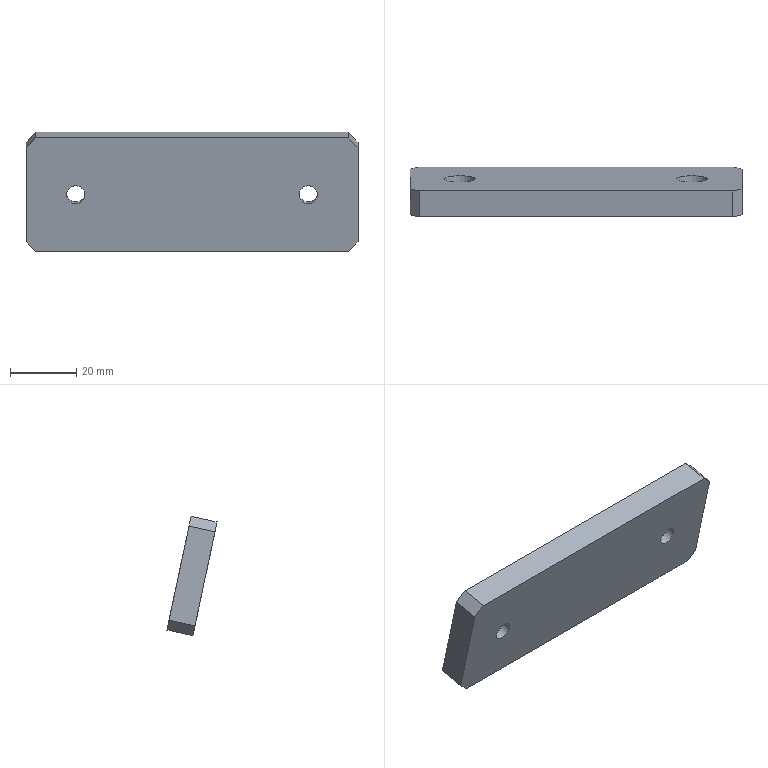Part | STEP file | P011002S001-005 | 1 solid | 16 faces | box 100 x 15.102 x 35.898 mm | volume 26958 mm3 | plane 12 | cylinder 4 | commonest cylinder face diameters 5.5 x2 9.5 x2
STEP:
#1=CARTESIAN_POINT('',(0.,0.,0.));
#2=DIRECTION('',(0.,0.,1.));
#3=DIRECTION('',(1.,0.,0.));
#4=AXIS2_PLACEMENT_3D('',#1,#2,#3);
#5=CARTESIAN_POINT('',(34.5,246.537,21.808));
#6=VERTEX_POINT('',#5);
#7=CARTESIAN_POINT('',(34.5,245.966,24.498));
#8=DIRECTION('',(0.,-0.9781,-0.2079));
#9=DIRECTION('',(0.,0.2079,-0.9781));
#10=AXIS2_PLACEMENT_3D('',#7,#8,#9);
#11=CIRCLE('',#10,2.75);
#12=CARTESIAN_POINT('',(-5.5,243.367,36.725));
#13=DIRECTION('',(0.,-0.9781,-0.2079));
#14=DIRECTION('',(1.,0.,0.));
#15=AXIS2_PLACEMENT_3D('',#12,#13,#14);
#16=PLANE('',#15);
#17=CARTESIAN_POINT('',(40.,-12.5));
#18=DIRECTION('',(0.,-1.));
#19=AXIS2_PLACEMENT_2D('',#17,#18);
#20=CIRCLE('',#19,2.75);
#21=(GEOMETRIC_REPRESENTATION_CONTEXT(2)PARAMETRIC_REPRESENTATION_CONTEXT()REPRESENTATION_CONTEXT('',''));
#22=DEFINITIONAL_REPRESENTATION('',(#20),#21);
#23=PCURVE('',#16,#22);
#24=CARTESIAN_POINT('',(34.5,253.791,26.161));
#25=DIRECTION('',(0.,-0.9781,-0.2079));
#26=DIRECTION('',(0.,0.2079,-0.9781));
#27=AXIS2_PLACEMENT_3D('',#24,#25,#26);
#28=CYLINDRICAL_SURFACE('',#27,2.75);
#29=CARTESIAN_POINT('',(0.,8.));
#30=DIRECTION('',(1.,0.));
#31=VECTOR('',#30,1.);
#32=LINE('',#29,#31);
#33=(GEOMETRIC_REPRESENTATION_CONTEXT(2)PARAMETRIC_REPRESENTATION_CONTEXT()REPRESENTATION_CONTEXT('',''));
#34=DEFINITIONAL_REPRESENTATION('',(#32),#33);
#35=PCURVE('',#28,#34);
#36=SURFACE_CURVE('',#11,(#23,#35),.PCURVE_S1.);
#37=EDGE_CURVE('',#6,#6,#36,.T.);
#38=ORIENTED_EDGE('',*,*,#37,.F.);
#39=EDGE_LOOP('',(#38));
#40=FACE_BOUND('',#39,.T.);
#41=CARTESIAN_POINT('',(49.5,248.98,10.315));
#42=VERTEX_POINT('',#41);
#43=CARTESIAN_POINT('',(49.5,242.951,38.681));
#44=VERTEX_POINT('',#43);
#45=CARTESIAN_POINT('',(49.5,259.129,-37.432));
#46=DIRECTION('',(0.,-0.2079,0.9781));
#47=VECTOR('',#46,1.);
#48=LINE('',#45,#47);
#49=CARTESIAN_POINT('',(55.,-75.813));
#50=DIRECTION('',(0.,1.));
#51=VECTOR('',#50,1.);
#52=LINE('',#49,#51);
#53=(GEOMETRIC_REPRESENTATION_CONTEXT(2)PARAMETRIC_REPRESENTATION_CONTEXT()REPRESENTATION_CONTEXT('',''));
#54=DEFINITIONAL_REPRESENTATION('',(#52),#53);
#55=PCURVE('',#16,#54);
#56=CARTESIAN_POINT('',(49.5,200.,-50.));
#57=DIRECTION('',(-1.,0.,0.));
#58=DIRECTION('',(0.,0.,1.));
#59=AXIS2_PLACEMENT_3D('',#56,#57,#58);
#60=PLANE('',#59);
#61=CARTESIAN_POINT('',(12.568,59.129));
#62=DIRECTION('',(0.9781,-0.2079));
#63=VECTOR('',#62,1.);
#64=LINE('',#61,#63);
#65=(GEOMETRIC_REPRESENTATION_CONTEXT(2)PARAMETRIC_REPRESENTATION_CONTEXT()REPRESENTATION_CONTEXT('',''));
#66=DEFINITIONAL_REPRESENTATION('',(#64),#65);
#67=PCURVE('',#60,#66);
#68=SURFACE_CURVE('',#48,(#55,#67),.PCURVE_S1.);
#69=EDGE_CURVE('',#42,#44,#68,.T.);
#70=ORIENTED_EDGE('',*,*,#69,.T.);
#71=CARTESIAN_POINT('',(46.5,242.327,41.615));
#72=VERTEX_POINT('',#71);
#73=CARTESIAN_POINT('',(23.,237.441,64.602));
#74=DIRECTION('',(0.7071,0.147,-0.6917));
#75=VECTOR('',#74,1.);
#76=LINE('',#73,#75);
#77=CARTESIAN_POINT('',(28.5,28.5));
#78=DIRECTION('',(0.7071,-0.7071));
#79=VECTOR('',#78,1.);
#80=LINE('',#77,#79);
#81=(GEOMETRIC_REPRESENTATION_CONTEXT(2)PARAMETRIC_REPRESENTATION_CONTEXT()REPRESENTATION_CONTEXT('',''));
#82=DEFINITIONAL_REPRESENTATION('',(#80),#81);
#83=PCURVE('',#16,#82);
#84=CARTESIAN_POINT('',(49.5,183.822,26.113));
#85=DIRECTION('',(0.7071,-0.147,0.6917));
#86=DIRECTION('',(-0.6993,0.,0.7149));
#87=AXIS2_PLACEMENT_3D('',#84,#85,#86);
#88=PLANE('',#87);
#89=CARTESIAN_POINT('',(46.045,-54.209));
#90=DIRECTION('',(-0.9889,-0.1486));
#91=VECTOR('',#90,1.);
#92=LINE('',#89,#91);
#93=(GEOMETRIC_REPRESENTATION_CONTEXT(2)PARAMETRIC_REPRESENTATION_CONTEXT()REPRESENTATION_CONTEXT('',''));
#94=DEFINITIONAL_REPRESENTATION('',(#92),#93);
#95=PCURVE('',#88,#94);
#96=SURFACE_CURVE('',#76,(#83,#95),.PCURVE_S1.);
#97=EDGE_CURVE('',#72,#44,#96,.T.);
#98=ORIENTED_EDGE('',*,*,#97,.F.);
#99=CARTESIAN_POINT('',(-47.5,242.327,41.615));
#100=VERTEX_POINT('',#99);
#101=CARTESIAN_POINT('',(-5.5,242.327,41.615));
#102=DIRECTION('',(-1.,0.,0.));
#103=VECTOR('',#102,1.);
#104=LINE('',#101,#103);
#105=CARTESIAN_POINT('',(0.,5.));
#106=DIRECTION('',(-1.,0.));
#107=VECTOR('',#106,1.);
#108=LINE('',#105,#107);
#109=(GEOMETRIC_REPRESENTATION_CONTEXT(2)PARAMETRIC_REPRESENTATION_CONTEXT()REPRESENTATION_CONTEXT('',''));
#110=DEFINITIONAL_REPRESENTATION('',(#108),#109);
#111=PCURVE('',#16,#110);
#112=CARTESIAN_POINT('',(-5.5,249.663,43.175));
#113=DIRECTION('',(0.,-0.2079,0.9781));
#114=DIRECTION('',(0.,-0.9781,-0.2079));
#115=AXIS2_PLACEMENT_3D('',#112,#113,#114);
#116=PLANE('',#115);
#117=CARTESIAN_POINT('',(7.5,0.));
#118=DIRECTION('',(0.,-1.));
#119=VECTOR('',#118,1.);
#120=LINE('',#117,#119);
#121=(GEOMETRIC_REPRESENTATION_CONTEXT(2)PARAMETRIC_REPRESENTATION_CONTEXT()REPRESENTATION_CONTEXT('',''));
#122=DEFINITIONAL_REPRESENTATION('',(#120),#121);
#123=PCURVE('',#116,#122);
#124=SURFACE_CURVE('',#104,(#111,#123),.PCURVE_S1.);
#125=EDGE_CURVE('',#72,#100,#124,.T.);
#126=ORIENTED_EDGE('',*,*,#125,.T.);
#127=CARTESIAN_POINT('',(-50.5,242.951,38.681));
#128=VERTEX_POINT('',#127);
#129=CARTESIAN_POINT('',(-29.,238.481,59.711));
#130=DIRECTION('',(0.7071,-0.147,0.6917));
#131=VECTOR('',#130,1.);
#132=LINE('',#129,#131);
#133=CARTESIAN_POINT('',(-23.5,23.5));
#134=DIRECTION('',(0.7071,0.7071));
#135=VECTOR('',#134,1.);
#136=LINE('',#133,#135);
#137=(GEOMETRIC_REPRESENTATION_CONTEXT(2)PARAMETRIC_REPRESENTATION_CONTEXT()REPRESENTATION_CONTEXT('',''));
#138=DEFINITIONAL_REPRESENTATION('',(#136),#137);
#139=PCURVE('',#16,#138);
#140=CARTESIAN_POINT('',(-47.5,249.663,43.175));
#141=DIRECTION('',(0.7071,0.147,-0.6917));
#142=DIRECTION('',(0.6993,0.,0.7149));
#143=AXIS2_PLACEMENT_3D('',#140,#141,#142);
#144=PLANE('',#143);
#145=CARTESIAN_POINT('',(24.758,11.305));
#146=DIRECTION('',(0.9889,0.1486));
#147=VECTOR('',#146,1.);
#148=LINE('',#145,#147);
#149=(GEOMETRIC_REPRESENTATION_CONTEXT(2)PARAMETRIC_REPRESENTATION_CONTEXT()REPRESENTATION_CONTEXT('',''));
#150=DEFINITIONAL_REPRESENTATION('',(#148),#149);
#151=PCURVE('',#144,#150);
#152=SURFACE_CURVE('',#132,(#139,#151),.PCURVE_S1.);
#153=EDGE_CURVE('',#128,#100,#152,.T.);
#154=ORIENTED_EDGE('',*,*,#153,.F.);
#155=CARTESIAN_POINT('',(-50.5,248.98,10.315));
#156=VERTEX_POINT('',#155);
#157=CARTESIAN_POINT('',(-50.5,259.129,-37.432));
#158=DIRECTION('',(0.,0.2079,-0.9781));
#159=VECTOR('',#158,1.);
#160=LINE('',#157,#159);
#161=CARTESIAN_POINT('',(-45.,-75.813));
#162=DIRECTION('',(0.,-1.));
#163=VECTOR('',#162,1.);
#164=LINE('',#161,#163);
#165=(GEOMETRIC_REPRESENTATION_CONTEXT(2)PARAMETRIC_REPRESENTATION_CONTEXT()REPRESENTATION_CONTEXT('',''));
#166=DEFINITIONAL_REPRESENTATION('',(#164),#165);
#167=PCURVE('',#16,#166);
#168=CARTESIAN_POINT('',(-50.5,200.,-50.));
#169=DIRECTION('',(-1.,0.,0.));
#170=DIRECTION('',(0.,0.,1.));
#171=AXIS2_PLACEMENT_3D('',#168,#169,#170);
#172=PLANE('',#171);
#173=CARTESIAN_POINT('',(12.568,59.129));
#174=DIRECTION('',(-0.9781,0.2079));
#175=VECTOR('',#174,1.);
#176=LINE('',#173,#175);
#177=(GEOMETRIC_REPRESENTATION_CONTEXT(2)PARAMETRIC_REPRESENTATION_CONTEXT()REPRESENTATION_CONTEXT('',''));
#178=DEFINITIONAL_REPRESENTATION('',(#176),#177);
#179=PCURVE('',#172,#178);
#180=SURFACE_CURVE('',#160,(#167,#179),.PCURVE_S1.);
#181=EDGE_CURVE('',#128,#156,#180,.T.);
#182=ORIENTED_EDGE('',*,*,#181,.T.);
#183=CARTESIAN_POINT('',(-47.5,249.604,7.38));
#184=VERTEX_POINT('',#183);
#185=CARTESIAN_POINT('',(-41.5,250.852,1.511));
#186=DIRECTION('',(-0.7071,-0.147,0.6917));
#187=VECTOR('',#186,1.);
#188=LINE('',#185,#187);
#189=CARTESIAN_POINT('',(-36.,-36.));
#190=DIRECTION('',(-0.7071,0.7071));
#191=VECTOR('',#190,1.);
#192=LINE('',#189,#191);
#193=(GEOMETRIC_REPRESENTATION_CONTEXT(2)PARAMETRIC_REPRESENTATION_CONTEXT()REPRESENTATION_CONTEXT('',''));
#194=DEFINITIONAL_REPRESENTATION('',(#192),#193);
#195=PCURVE('',#16,#194);
#196=CARTESIAN_POINT('',(-50.5,189.851,-2.254));
#197=DIRECTION('',(0.7071,-0.147,0.6917));
#198=DIRECTION('',(-0.6993,0.,0.7149));
#199=AXIS2_PLACEMENT_3D('',#196,#197,#198);
#200=PLANE('',#199);
#201=CARTESIAN_POINT('',(-3.602,-61.67));
#202=DIRECTION('',(0.9889,0.1486));
#203=VECTOR('',#202,1.);
#204=LINE('',#201,#203);
#205=(GEOMETRIC_REPRESENTATION_CONTEXT(2)PARAMETRIC_REPRESENTATION_CONTEXT()REPRESENTATION_CONTEXT('',''));
#206=DEFINITIONAL_REPRESENTATION('',(#204),#205);
#207=PCURVE('',#200,#206);
#208=SURFACE_CURVE('',#188,(#195,#207),.PCURVE_S1.);
#209=EDGE_CURVE('',#184,#156,#208,.T.);
#210=ORIENTED_EDGE('',*,*,#209,.F.);
#211=CARTESIAN_POINT('',(46.5,249.604,7.38));
#212=VERTEX_POINT('',#211);
#213=CARTESIAN_POINT('',(-5.5,249.604,7.38));
#214=DIRECTION('',(1.,0.,0.));
#215=VECTOR('',#214,1.);
#216=LINE('',#213,#215);
#217=CARTESIAN_POINT('',(0.,-30.));
#218=DIRECTION('',(1.,0.));
#219=VECTOR('',#218,1.);
#220=LINE('',#217,#219);
#221=(GEOMETRIC_REPRESENTATION_CONTEXT(2)PARAMETRIC_REPRESENTATION_CONTEXT()REPRESENTATION_CONTEXT('',''));
#222=DEFINITIONAL_REPRESENTATION('',(#220),#221);
#223=PCURVE('',#16,#222);
#224=CARTESIAN_POINT('',(-5.5,256.94,8.94));
#225=DIRECTION('',(0.,0.2079,-0.9781));
#226=DIRECTION('',(0.,0.9781,0.2079));
#227=AXIS2_PLACEMENT_3D('',#224,#225,#226);
#228=PLANE('',#227);
#229=CARTESIAN_POINT('',(-7.5,0.));
#230=DIRECTION('',(0.,1.));
#231=VECTOR('',#230,1.);
#232=LINE('',#229,#231);
#233=(GEOMETRIC_REPRESENTATION_CONTEXT(2)PARAMETRIC_REPRESENTATION_CONTEXT()REPRESENTATION_CONTEXT('',''));
#234=DEFINITIONAL_REPRESENTATION('',(#232),#233);
#235=PCURVE('',#228,#234);
#236=SURFACE_CURVE('',#216,(#223,#235),.PCURVE_S1.);
#237=EDGE_CURVE('',#184,#212,#236,.T.);
#238=ORIENTED_EDGE('',*,*,#237,.T.);
#239=CARTESIAN_POINT('',(35.5,251.891,-3.379));
#240=DIRECTION('',(-0.7071,0.147,-0.6917));
#241=VECTOR('',#240,1.);
#242=LINE('',#239,#241);
#243=CARTESIAN_POINT('',(41.,-41.));
#244=DIRECTION('',(-0.7071,-0.7071));
#245=VECTOR('',#244,1.);
#246=LINE('',#243,#245);
#247=(GEOMETRIC_REPRESENTATION_CONTEXT(2)PARAMETRIC_REPRESENTATION_CONTEXT()REPRESENTATION_CONTEXT('',''));
#248=DEFINITIONAL_REPRESENTATION('',(#246),#247);
#249=PCURVE('',#16,#248);
#250=CARTESIAN_POINT('',(46.5,256.94,8.94));
#251=DIRECTION('',(0.7071,0.147,-0.6917));
#252=DIRECTION('',(0.6993,0.,0.7149));
#253=AXIS2_PLACEMENT_3D('',#250,#251,#252);
#254=PLANE('',#253);
#255=CARTESIAN_POINT('',(-16.498,5.105));
#256=DIRECTION('',(-0.9889,-0.1486));
#257=VECTOR('',#256,1.);
#258=LINE('',#255,#257);
#259=(GEOMETRIC_REPRESENTATION_CONTEXT(2)PARAMETRIC_REPRESENTATION_CONTEXT()REPRESENTATION_CONTEXT('',''));
#260=DEFINITIONAL_REPRESENTATION('',(#258),#259);
#261=PCURVE('',#254,#260);
#262=SURFACE_CURVE('',#242,(#249,#261),.PCURVE_S1.);
#263=EDGE_CURVE('',#42,#212,#262,.T.);
#264=ORIENTED_EDGE('',*,*,#263,.F.);
#265=EDGE_LOOP('',(#70,#98,#126,#154,#182,#210,#238,#264));
#266=FACE_BOUND('',#265,.T.);
#267=CARTESIAN_POINT('',(-35.5,246.537,21.808));
#268=VERTEX_POINT('',#267);
#269=CARTESIAN_POINT('',(-35.5,245.966,24.498));
#270=DIRECTION('',(0.,-0.9781,-0.2079));
#271=DIRECTION('',(0.,0.2079,-0.9781));
#272=AXIS2_PLACEMENT_3D('',#269,#270,#271);
#273=CIRCLE('',#272,2.75);
#274=CARTESIAN_POINT('',(-30.,-12.5));
#275=DIRECTION('',(0.,-1.));
#276=AXIS2_PLACEMENT_2D('',#274,#275);
#277=CIRCLE('',#276,2.75);
#278=(GEOMETRIC_REPRESENTATION_CONTEXT(2)PARAMETRIC_REPRESENTATION_CONTEXT()REPRESENTATION_CONTEXT('',''));
#279=DEFINITIONAL_REPRESENTATION('',(#277),#278);
#280=PCURVE('',#16,#279);
#281=CARTESIAN_POINT('',(-35.5,253.791,26.161));
#282=DIRECTION('',(0.,-0.9781,-0.2079));
#283=DIRECTION('',(0.,0.2079,-0.9781));
#284=AXIS2_PLACEMENT_3D('',#281,#282,#283);
#285=CYLINDRICAL_SURFACE('',#284,2.75);
#286=CARTESIAN_POINT('',(0.,8.));
#287=DIRECTION('',(1.,0.));
#288=VECTOR('',#287,1.);
#289=LINE('',#286,#288);
#290=(GEOMETRIC_REPRESENTATION_CONTEXT(2)PARAMETRIC_REPRESENTATION_CONTEXT()REPRESENTATION_CONTEXT('',''));
#291=DEFINITIONAL_REPRESENTATION('',(#289),#290);
#292=PCURVE('',#285,#291);
#293=SURFACE_CURVE('',#273,(#280,#292),.PCURVE_S1.);
#294=EDGE_CURVE('',#268,#268,#293,.T.);
#295=ORIENTED_EDGE('',*,*,#294,.F.);
#296=EDGE_LOOP('',(#295));
#297=FACE_BOUND('',#296,.T.);
#298=ADVANCED_FACE('',(#40,#266,#297),#16,.T.);
#299=CARTESIAN_POINT('',(-35.5,254.778,21.515));
#300=VERTEX_POINT('',#299);
#301=CARTESIAN_POINT('',(-35.5,253.791,26.161));
#302=DIRECTION('',(0.,-0.9781,-0.2079));
#303=DIRECTION('',(0.,0.2079,-0.9781));
#304=AXIS2_PLACEMENT_3D('',#301,#302,#303);
#305=CIRCLE('',#304,4.75);
#306=CARTESIAN_POINT('',(-5.5,251.192,38.388));
#307=DIRECTION('',(0.,0.9781,0.2079));
#308=DIRECTION('',(-1.,0.,0.));
#309=AXIS2_PLACEMENT_3D('',#306,#307,#308);
#310=PLANE('',#309);
#311=CARTESIAN_POINT('',(30.,-17.25));
#312=CARTESIAN_POINT('',(21.773,-17.25));
#313=CARTESIAN_POINT('',(25.886,-10.125));
#314=CARTESIAN_POINT('',(30.,-3.));
#315=CARTESIAN_POINT('',(34.114,-10.125));
#316=CARTESIAN_POINT('',(38.227,-17.25));
#317=CARTESIAN_POINT('',(30.,-17.25));
#318=(BOUNDED_CURVE()B_SPLINE_CURVE(2,(#311,#312,#313,#314,#315,#316,#317),.UNSPECIFIED.,.T.,.F.)B_SPLINE_CURVE_WITH_KNOTS((1,2,2,2,2,1),(-2.094,0.,2.094,4.189,6.283,8.378),.UNSPECIFIED.)CURVE()GEOMETRIC_REPRESENTATION_ITEM()RATIONAL_B_SPLINE_CURVE((1.,0.5,1.,0.5,1.,0.5,1.))REPRESENTATION_ITEM(''));
#319=(GEOMETRIC_REPRESENTATION_CONTEXT(2)PARAMETRIC_REPRESENTATION_CONTEXT()REPRESENTATION_CONTEXT('',''));
#320=DEFINITIONAL_REPRESENTATION('',(#318),#319);
#321=PCURVE('',#310,#320);
#322=CARTESIAN_POINT('',(-35.5,253.791,26.161));
#323=DIRECTION('',(0.,-0.9781,-0.2079));
#324=DIRECTION('',(0.,0.2079,-0.9781));
#325=AXIS2_PLACEMENT_3D('',#322,#323,#324);
#326=CYLINDRICAL_SURFACE('',#325,4.75);
#327=CARTESIAN_POINT('',(0.,0.));
#328=DIRECTION('',(1.,0.));
#329=VECTOR('',#328,1.);
#330=LINE('',#327,#329);
#331=(GEOMETRIC_REPRESENTATION_CONTEXT(2)PARAMETRIC_REPRESENTATION_CONTEXT()REPRESENTATION_CONTEXT('',''));
#332=DEFINITIONAL_REPRESENTATION('',(#330),#331);
#333=PCURVE('',#326,#332);
#334=SURFACE_CURVE('',#305,(#321,#333),.PCURVE_S1.);
#335=EDGE_CURVE('',#300,#300,#334,.T.);
#336=ORIENTED_EDGE('',*,*,#335,.T.);
#337=EDGE_LOOP('',(#336));
#338=FACE_BOUND('',#337,.T.);
#339=CARTESIAN_POINT('',(34.5,254.778,21.515));
#340=VERTEX_POINT('',#339);
#341=CARTESIAN_POINT('',(34.5,253.791,26.161));
#342=DIRECTION('',(0.,-0.9781,-0.2079));
#343=DIRECTION('',(0.,0.2079,-0.9781));
#344=AXIS2_PLACEMENT_3D('',#341,#342,#343);
#345=CIRCLE('',#344,4.75);
#346=CARTESIAN_POINT('',(-40.,-17.25));
#347=CARTESIAN_POINT('',(-48.227,-17.25));
#348=CARTESIAN_POINT('',(-44.114,-10.125));
#349=CARTESIAN_POINT('',(-40.,-3.));
#350=CARTESIAN_POINT('',(-35.886,-10.125));
#351=CARTESIAN_POINT('',(-31.773,-17.25));
#352=CARTESIAN_POINT('',(-40.,-17.25));
#353=(BOUNDED_CURVE()B_SPLINE_CURVE(2,(#346,#347,#348,#349,#350,#351,#352),.UNSPECIFIED.,.T.,.F.)B_SPLINE_CURVE_WITH_KNOTS((1,2,2,2,2,1),(-2.094,0.,2.094,4.189,6.283,8.378),.UNSPECIFIED.)CURVE()GEOMETRIC_REPRESENTATION_ITEM()RATIONAL_B_SPLINE_CURVE((1.,0.5,1.,0.5,1.,0.5,1.))REPRESENTATION_ITEM(''));
#354=(GEOMETRIC_REPRESENTATION_CONTEXT(2)PARAMETRIC_REPRESENTATION_CONTEXT()REPRESENTATION_CONTEXT('',''));
#355=DEFINITIONAL_REPRESENTATION('',(#353),#354);
#356=PCURVE('',#310,#355);
#357=CARTESIAN_POINT('',(34.5,253.791,26.161));
#358=DIRECTION('',(0.,-0.9781,-0.2079));
#359=DIRECTION('',(0.,0.2079,-0.9781));
#360=AXIS2_PLACEMENT_3D('',#357,#358,#359);
#361=CYLINDRICAL_SURFACE('',#360,4.75);
#362=CARTESIAN_POINT('',(0.,0.));
#363=DIRECTION('',(1.,0.));
#364=VECTOR('',#363,1.);
#365=LINE('',#362,#364);
#366=(GEOMETRIC_REPRESENTATION_CONTEXT(2)PARAMETRIC_REPRESENTATION_CONTEXT()REPRESENTATION_CONTEXT('',''));
#367=DEFINITIONAL_REPRESENTATION('',(#365),#366);
#368=PCURVE('',#361,#367);
#369=SURFACE_CURVE('',#345,(#356,#368),.PCURVE_S1.);
#370=EDGE_CURVE('',#340,#340,#369,.T.);
#371=ORIENTED_EDGE('',*,*,#370,.T.);
#372=EDGE_LOOP('',(#371));
#373=FACE_BOUND('',#372,.T.);
#374=CARTESIAN_POINT('',(46.5,257.429,9.044));
#375=VERTEX_POINT('',#374);
#376=CARTESIAN_POINT('',(-47.5,257.429,9.044));
#377=VERTEX_POINT('',#376);
#378=CARTESIAN_POINT('',(-5.5,257.429,9.044));
#379=DIRECTION('',(-1.,0.,0.));
#380=VECTOR('',#379,1.);
#381=LINE('',#378,#380);
#382=CARTESIAN_POINT('',(0.,-30.));
#383=DIRECTION('',(1.,0.));
#384=VECTOR('',#383,1.);
#385=LINE('',#382,#384);
#386=(GEOMETRIC_REPRESENTATION_CONTEXT(2)PARAMETRIC_REPRESENTATION_CONTEXT()REPRESENTATION_CONTEXT('',''));
#387=DEFINITIONAL_REPRESENTATION('',(#385),#386);
#388=PCURVE('',#310,#387);
#389=CARTESIAN_POINT('',(0.5,0.));
#390=DIRECTION('',(0.,-1.));
#391=VECTOR('',#390,1.);
#392=LINE('',#389,#391);
#393=(GEOMETRIC_REPRESENTATION_CONTEXT(2)PARAMETRIC_REPRESENTATION_CONTEXT()REPRESENTATION_CONTEXT('',''));
#394=DEFINITIONAL_REPRESENTATION('',(#392),#393);
#395=PCURVE('',#228,#394);
#396=SURFACE_CURVE('',#381,(#388,#395),.PCURVE_S1.);
#397=EDGE_CURVE('',#375,#377,#396,.T.);
#398=ORIENTED_EDGE('',*,*,#397,.T.);
#399=CARTESIAN_POINT('',(-50.5,256.806,11.978));
#400=VERTEX_POINT('',#399);
#401=CARTESIAN_POINT('',(-41.5,258.677,3.175));
#402=DIRECTION('',(0.7071,0.147,-0.6917));
#403=VECTOR('',#402,1.);
#404=LINE('',#401,#403);
#405=CARTESIAN_POINT('',(36.,-36.));
#406=DIRECTION('',(-0.7071,-0.7071));
#407=VECTOR('',#406,1.);
#408=LINE('',#405,#407);
#409=(GEOMETRIC_REPRESENTATION_CONTEXT(2)PARAMETRIC_REPRESENTATION_CONTEXT()REPRESENTATION_CONTEXT('',''));
#410=DEFINITIONAL_REPRESENTATION('',(#408),#409);
#411=PCURVE('',#310,#410);
#412=CARTESIAN_POINT('',(-2.413,-69.582));
#413=DIRECTION('',(-0.9889,-0.1486));
#414=VECTOR('',#413,1.);
#415=LINE('',#412,#414);
#416=(GEOMETRIC_REPRESENTATION_CONTEXT(2)PARAMETRIC_REPRESENTATION_CONTEXT()REPRESENTATION_CONTEXT('',''));
#417=DEFINITIONAL_REPRESENTATION('',(#415),#416);
#418=PCURVE('',#200,#417);
#419=SURFACE_CURVE('',#404,(#411,#418),.PCURVE_S1.);
#420=EDGE_CURVE('',#400,#377,#419,.T.);
#421=ORIENTED_EDGE('',*,*,#420,.F.);
#422=CARTESIAN_POINT('',(-50.5,250.776,40.344));
#423=VERTEX_POINT('',#422);
#424=CARTESIAN_POINT('',(-50.5,266.954,-35.768));
#425=DIRECTION('',(0.,-0.2079,0.9781));
#426=VECTOR('',#425,1.);
#427=LINE('',#424,#426);
#428=CARTESIAN_POINT('',(45.,-75.813));
#429=DIRECTION('',(0.,1.));
#430=VECTOR('',#429,1.);
#431=LINE('',#428,#430);
#432=(GEOMETRIC_REPRESENTATION_CONTEXT(2)PARAMETRIC_REPRESENTATION_CONTEXT()REPRESENTATION_CONTEXT('',''));
#433=DEFINITIONAL_REPRESENTATION('',(#431),#432);
#434=PCURVE('',#310,#433);
#435=CARTESIAN_POINT('',(14.232,66.954));
#436=DIRECTION('',(0.9781,-0.2079));
#437=VECTOR('',#436,1.);
#438=LINE('',#435,#437);
#439=(GEOMETRIC_REPRESENTATION_CONTEXT(2)PARAMETRIC_REPRESENTATION_CONTEXT()REPRESENTATION_CONTEXT('',''));
#440=DEFINITIONAL_REPRESENTATION('',(#438),#439);
#441=PCURVE('',#172,#440);
#442=SURFACE_CURVE('',#427,(#434,#441),.PCURVE_S1.);
#443=EDGE_CURVE('',#400,#423,#442,.T.);
#444=ORIENTED_EDGE('',*,*,#443,.T.);
#445=CARTESIAN_POINT('',(-47.5,250.152,43.279));
#446=VERTEX_POINT('',#445);
#447=CARTESIAN_POINT('',(-29.,246.306,61.375));
#448=DIRECTION('',(-0.7071,0.147,-0.6917));
#449=VECTOR('',#448,1.);
#450=LINE('',#447,#449);
#451=CARTESIAN_POINT('',(23.5,23.5));
#452=DIRECTION('',(0.7071,-0.7071));
#453=VECTOR('',#452,1.);
#454=LINE('',#451,#453);
#455=(GEOMETRIC_REPRESENTATION_CONTEXT(2)PARAMETRIC_REPRESENTATION_CONTEXT()REPRESENTATION_CONTEXT('',''));
#456=DEFINITIONAL_REPRESENTATION('',(#454),#455);
#457=PCURVE('',#310,#456);
#458=CARTESIAN_POINT('',(25.947,3.394));
#459=DIRECTION('',(-0.9889,-0.1486));
#460=VECTOR('',#459,1.);
#461=LINE('',#458,#460);
#462=(GEOMETRIC_REPRESENTATION_CONTEXT(2)PARAMETRIC_REPRESENTATION_CONTEXT()REPRESENTATION_CONTEXT('',''));
#463=DEFINITIONAL_REPRESENTATION('',(#461),#462);
#464=PCURVE('',#144,#463);
#465=SURFACE_CURVE('',#450,(#457,#464),.PCURVE_S1.);
#466=EDGE_CURVE('',#446,#423,#465,.T.);
#467=ORIENTED_EDGE('',*,*,#466,.F.);
#468=CARTESIAN_POINT('',(46.5,250.152,43.279));
#469=VERTEX_POINT('',#468);
#470=CARTESIAN_POINT('',(-5.5,250.152,43.279));
#471=DIRECTION('',(1.,0.,0.));
#472=VECTOR('',#471,1.);
#473=LINE('',#470,#472);
#474=CARTESIAN_POINT('',(0.,5.));
#475=DIRECTION('',(-1.,0.));
#476=VECTOR('',#475,1.);
#477=LINE('',#474,#476);
#478=(GEOMETRIC_REPRESENTATION_CONTEXT(2)PARAMETRIC_REPRESENTATION_CONTEXT()REPRESENTATION_CONTEXT('',''));
#479=DEFINITIONAL_REPRESENTATION('',(#477),#478);
#480=PCURVE('',#310,#479);
#481=CARTESIAN_POINT('',(-0.5,0.));
#482=DIRECTION('',(0.,1.));
#483=VECTOR('',#482,1.);
#484=LINE('',#481,#483);
#485=(GEOMETRIC_REPRESENTATION_CONTEXT(2)PARAMETRIC_REPRESENTATION_CONTEXT()REPRESENTATION_CONTEXT('',''));
#486=DEFINITIONAL_REPRESENTATION('',(#484),#485);
#487=PCURVE('',#116,#486);
#488=SURFACE_CURVE('',#473,(#480,#487),.PCURVE_S1.);
#489=EDGE_CURVE('',#446,#469,#488,.T.);
#490=ORIENTED_EDGE('',*,*,#489,.T.);
#491=CARTESIAN_POINT('',(49.5,250.776,40.344));
#492=VERTEX_POINT('',#491);
#493=CARTESIAN_POINT('',(23.,245.266,66.265));
#494=DIRECTION('',(-0.7071,-0.147,0.6917));
#495=VECTOR('',#494,1.);
#496=LINE('',#493,#495);
#497=CARTESIAN_POINT('',(-28.5,28.5));
#498=DIRECTION('',(0.7071,0.7071));
#499=VECTOR('',#498,1.);
#500=LINE('',#497,#499);
#501=(GEOMETRIC_REPRESENTATION_CONTEXT(2)PARAMETRIC_REPRESENTATION_CONTEXT()REPRESENTATION_CONTEXT('',''));
#502=DEFINITIONAL_REPRESENTATION('',(#500),#501);
#503=PCURVE('',#310,#502);
#504=CARTESIAN_POINT('',(47.234,-62.12));
#505=DIRECTION('',(0.9889,0.1486));
#506=VECTOR('',#505,1.);
#507=LINE('',#504,#506);
#508=(GEOMETRIC_REPRESENTATION_CONTEXT(2)PARAMETRIC_REPRESENTATION_CONTEXT()REPRESENTATION_CONTEXT('',''));
#509=DEFINITIONAL_REPRESENTATION('',(#507),#508);
#510=PCURVE('',#88,#509);
#511=SURFACE_CURVE('',#496,(#503,#510),.PCURVE_S1.);
#512=EDGE_CURVE('',#492,#469,#511,.T.);
#513=ORIENTED_EDGE('',*,*,#512,.F.);
#514=CARTESIAN_POINT('',(49.5,256.806,11.978));
#515=VERTEX_POINT('',#514);
#516=CARTESIAN_POINT('',(49.5,266.954,-35.768));
#517=DIRECTION('',(0.,0.2079,-0.9781));
#518=VECTOR('',#517,1.);
#519=LINE('',#516,#518);
#520=CARTESIAN_POINT('',(-55.,-75.813));
#521=DIRECTION('',(0.,-1.));
#522=VECTOR('',#521,1.);
#523=LINE('',#520,#522);
#524=(GEOMETRIC_REPRESENTATION_CONTEXT(2)PARAMETRIC_REPRESENTATION_CONTEXT()REPRESENTATION_CONTEXT('',''));
#525=DEFINITIONAL_REPRESENTATION('',(#523),#524);
#526=PCURVE('',#310,#525);
#527=CARTESIAN_POINT('',(14.232,66.954));
#528=DIRECTION('',(-0.9781,0.2079));
#529=VECTOR('',#528,1.);
#530=LINE('',#527,#529);
#531=(GEOMETRIC_REPRESENTATION_CONTEXT(2)PARAMETRIC_REPRESENTATION_CONTEXT()REPRESENTATION_CONTEXT('',''));
#532=DEFINITIONAL_REPRESENTATION('',(#530),#531);
#533=PCURVE('',#60,#532);
#534=SURFACE_CURVE('',#519,(#526,#533),.PCURVE_S1.);
#535=EDGE_CURVE('',#492,#515,#534,.T.);
#536=ORIENTED_EDGE('',*,*,#535,.T.);
#537=CARTESIAN_POINT('',(35.5,259.716,-1.716));
#538=DIRECTION('',(0.7071,-0.147,0.6917));
#539=VECTOR('',#538,1.);
#540=LINE('',#537,#539);
#541=CARTESIAN_POINT('',(-41.,-41.));
#542=DIRECTION('',(-0.7071,0.7071));
#543=VECTOR('',#542,1.);
#544=LINE('',#541,#543);
#545=(GEOMETRIC_REPRESENTATION_CONTEXT(2)PARAMETRIC_REPRESENTATION_CONTEXT()REPRESENTATION_CONTEXT('',''));
#546=DEFINITIONAL_REPRESENTATION('',(#544),#545);
#547=PCURVE('',#310,#546);
#548=CARTESIAN_POINT('',(-15.309,-2.807));
#549=DIRECTION('',(0.9889,0.1486));
#550=VECTOR('',#549,1.);
#551=LINE('',#548,#550);
#552=(GEOMETRIC_REPRESENTATION_CONTEXT(2)PARAMETRIC_REPRESENTATION_CONTEXT()REPRESENTATION_CONTEXT('',''));
#553=DEFINITIONAL_REPRESENTATION('',(#551),#552);
#554=PCURVE('',#254,#553);
#555=SURFACE_CURVE('',#540,(#547,#554),.PCURVE_S1.);
#556=EDGE_CURVE('',#375,#515,#555,.T.);
#557=ORIENTED_EDGE('',*,*,#556,.F.);
#558=EDGE_LOOP('',(#398,#421,#444,#467,#490,#513,#536,#557));
#559=FACE_BOUND('',#558,.T.);
#560=ADVANCED_FACE('',(#338,#373,#559),#310,.T.);
#561=ORIENTED_EDGE('',*,*,#489,.F.);
#562=CARTESIAN_POINT('',(-47.5,249.663,43.175));
#563=DIRECTION('',(0.,0.9781,0.2079));
#564=VECTOR('',#563,1.);
#565=LINE('',#562,#564);
#566=CARTESIAN_POINT('',(0.,-42.));
#567=DIRECTION('',(-1.,0.));
#568=VECTOR('',#567,1.);
#569=LINE('',#566,#568);
#570=(GEOMETRIC_REPRESENTATION_CONTEXT(2)PARAMETRIC_REPRESENTATION_CONTEXT()REPRESENTATION_CONTEXT('',''));
#571=DEFINITIONAL_REPRESENTATION('',(#569),#570);
#572=PCURVE('',#116,#571);
#573=CARTESIAN_POINT('',(0.,0.));
#574=DIRECTION('',(0.1486,-0.9889));
#575=VECTOR('',#574,1.);
#576=LINE('',#573,#575);
#577=(GEOMETRIC_REPRESENTATION_CONTEXT(2)PARAMETRIC_REPRESENTATION_CONTEXT()REPRESENTATION_CONTEXT('',''));
#578=DEFINITIONAL_REPRESENTATION('',(#576),#577);
#579=PCURVE('',#144,#578);
#580=SURFACE_CURVE('',#565,(#572,#579),.PCURVE_S1.);
#581=EDGE_CURVE('',#100,#446,#580,.T.);
#582=ORIENTED_EDGE('',*,*,#581,.F.);
#583=ORIENTED_EDGE('',*,*,#125,.F.);
#584=CARTESIAN_POINT('',(46.5,249.663,43.175));
#585=DIRECTION('',(0.,-0.9781,-0.2079));
#586=VECTOR('',#585,1.);
#587=LINE('',#584,#586);
#588=CARTESIAN_POINT('',(0.,52.));
#589=DIRECTION('',(1.,0.));
#590=VECTOR('',#589,1.);
#591=LINE('',#588,#590);
#592=(GEOMETRIC_REPRESENTATION_CONTEXT(2)PARAMETRIC_REPRESENTATION_CONTEXT()REPRESENTATION_CONTEXT('',''));
#593=DEFINITIONAL_REPRESENTATION('',(#591),#592);
#594=PCURVE('',#116,#593);
#595=CARTESIAN_POINT('',(14.295,-66.565));
#596=DIRECTION('',(-0.1486,0.9889));
#597=VECTOR('',#596,1.);
#598=LINE('',#595,#597);
#599=(GEOMETRIC_REPRESENTATION_CONTEXT(2)PARAMETRIC_REPRESENTATION_CONTEXT()REPRESENTATION_CONTEXT('',''));
#600=DEFINITIONAL_REPRESENTATION('',(#598),#599);
#601=PCURVE('',#88,#600);
#602=SURFACE_CURVE('',#587,(#594,#601),.PCURVE_S1.);
#603=EDGE_CURVE('',#469,#72,#602,.T.);
#604=ORIENTED_EDGE('',*,*,#603,.F.);
#605=EDGE_LOOP('',(#561,#582,#583,#604));
#606=FACE_BOUND('',#605,.T.);
#607=ADVANCED_FACE('',(#606),#116,.T.);
#608=ORIENTED_EDGE('',*,*,#535,.F.);
#609=CARTESIAN_POINT('',(49.5,183.822,26.113));
#610=DIRECTION('',(0.,0.9781,0.2079));
#611=VECTOR('',#610,1.);
#612=LINE('',#609,#611);
#613=CARTESIAN_POINT('',(76.113,-16.178));
#614=DIRECTION('',(0.2079,0.9781));
#615=VECTOR('',#614,1.);
#616=LINE('',#613,#615);
#617=(GEOMETRIC_REPRESENTATION_CONTEXT(2)PARAMETRIC_REPRESENTATION_CONTEXT()REPRESENTATION_CONTEXT('',''));
#618=DEFINITIONAL_REPRESENTATION('',(#616),#617);
#619=PCURVE('',#60,#618);
#620=CARTESIAN_POINT('',(0.,0.));
#621=DIRECTION('',(0.1486,-0.9889));
#622=VECTOR('',#621,1.);
#623=LINE('',#620,#622);
#624=(GEOMETRIC_REPRESENTATION_CONTEXT(2)PARAMETRIC_REPRESENTATION_CONTEXT()REPRESENTATION_CONTEXT('',''));
#625=DEFINITIONAL_REPRESENTATION('',(#623),#624);
#626=PCURVE('',#88,#625);
#627=SURFACE_CURVE('',#612,(#619,#626),.PCURVE_S1.);
#628=EDGE_CURVE('',#44,#492,#627,.T.);
#629=ORIENTED_EDGE('',*,*,#628,.F.);
#630=ORIENTED_EDGE('',*,*,#69,.F.);
#631=CARTESIAN_POINT('',(49.5,189.851,-2.254));
#632=DIRECTION('',(0.,-0.9781,-0.2079));
#633=VECTOR('',#632,1.);
#634=LINE('',#631,#633);
#635=CARTESIAN_POINT('',(47.746,-10.149));
#636=DIRECTION('',(-0.2079,-0.9781));
#637=VECTOR('',#636,1.);
#638=LINE('',#635,#637);
#639=(GEOMETRIC_REPRESENTATION_CONTEXT(2)PARAMETRIC_REPRESENTATION_CONTEXT()REPRESENTATION_CONTEXT('',''));
#640=DEFINITIONAL_REPRESENTATION('',(#638),#639);
#641=PCURVE('',#60,#640);
#642=CARTESIAN_POINT('',(-5.904,67.826));
#643=DIRECTION('',(-0.1486,0.9889));
#644=VECTOR('',#643,1.);
#645=LINE('',#642,#644);
#646=(GEOMETRIC_REPRESENTATION_CONTEXT(2)PARAMETRIC_REPRESENTATION_CONTEXT()REPRESENTATION_CONTEXT('',''));
#647=DEFINITIONAL_REPRESENTATION('',(#645),#646);
#648=PCURVE('',#254,#647);
#649=SURFACE_CURVE('',#634,(#641,#648),.PCURVE_S1.);
#650=EDGE_CURVE('',#515,#42,#649,.T.);
#651=ORIENTED_EDGE('',*,*,#650,.F.);
#652=EDGE_LOOP('',(#608,#629,#630,#651));
#653=FACE_BOUND('',#652,.T.);
#654=ADVANCED_FACE('',(#653),#60,.F.);
#655=ORIENTED_EDGE('',*,*,#237,.F.);
#656=CARTESIAN_POINT('',(-47.5,256.94,8.94));
#657=DIRECTION('',(0.,-0.9781,-0.2079));
#658=VECTOR('',#657,1.);
#659=LINE('',#656,#658);
#660=CARTESIAN_POINT('',(0.,-42.));
#661=DIRECTION('',(-1.,0.));
#662=VECTOR('',#661,1.);
#663=LINE('',#660,#662);
#664=(GEOMETRIC_REPRESENTATION_CONTEXT(2)PARAMETRIC_REPRESENTATION_CONTEXT()REPRESENTATION_CONTEXT('',''));
#665=DEFINITIONAL_REPRESENTATION('',(#663),#664);
#666=PCURVE('',#228,#665);
#667=CARTESIAN_POINT('',(5.904,-67.826));
#668=DIRECTION('',(-0.1486,0.9889));
#669=VECTOR('',#668,1.);
#670=LINE('',#667,#669);
#671=(GEOMETRIC_REPRESENTATION_CONTEXT(2)PARAMETRIC_REPRESENTATION_CONTEXT()REPRESENTATION_CONTEXT('',''));
#672=DEFINITIONAL_REPRESENTATION('',(#670),#671);
#673=PCURVE('',#200,#672);
#674=SURFACE_CURVE('',#659,(#666,#673),.PCURVE_S1.);
#675=EDGE_CURVE('',#377,#184,#674,.T.);
#676=ORIENTED_EDGE('',*,*,#675,.F.);
#677=ORIENTED_EDGE('',*,*,#397,.F.);
#678=CARTESIAN_POINT('',(46.5,256.94,8.94));
#679=DIRECTION('',(0.,0.9781,0.2079));
#680=VECTOR('',#679,1.);
#681=LINE('',#678,#680);
#682=CARTESIAN_POINT('',(0.,52.));
#683=DIRECTION('',(1.,0.));
#684=VECTOR('',#683,1.);
#685=LINE('',#682,#684);
#686=(GEOMETRIC_REPRESENTATION_CONTEXT(2)PARAMETRIC_REPRESENTATION_CONTEXT()REPRESENTATION_CONTEXT('',''));
#687=DEFINITIONAL_REPRESENTATION('',(#685),#686);
#688=PCURVE('',#228,#687);
#689=CARTESIAN_POINT('',(0.,0.));
#690=DIRECTION('',(0.1486,-0.9889));
#691=VECTOR('',#690,1.);
#692=LINE('',#689,#691);
#693=(GEOMETRIC_REPRESENTATION_CONTEXT(2)PARAMETRIC_REPRESENTATION_CONTEXT()REPRESENTATION_CONTEXT('',''));
#694=DEFINITIONAL_REPRESENTATION('',(#692),#693);
#695=PCURVE('',#254,#694);
#696=SURFACE_CURVE('',#681,(#688,#695),.PCURVE_S1.);
#697=EDGE_CURVE('',#212,#375,#696,.T.);
#698=ORIENTED_EDGE('',*,*,#697,.F.);
#699=EDGE_LOOP('',(#655,#676,#677,#698));
#700=FACE_BOUND('',#699,.T.);
#701=ADVANCED_FACE('',(#700),#228,.T.);
#702=ORIENTED_EDGE('',*,*,#181,.F.);
#703=CARTESIAN_POINT('',(-50.5,183.822,26.113));
#704=DIRECTION('',(0.,-0.9781,-0.2079));
#705=VECTOR('',#704,1.);
#706=LINE('',#703,#705);
#707=CARTESIAN_POINT('',(76.113,-16.178));
#708=DIRECTION('',(-0.2079,-0.9781));
#709=VECTOR('',#708,1.);
#710=LINE('',#707,#709);
#711=(GEOMETRIC_REPRESENTATION_CONTEXT(2)PARAMETRIC_REPRESENTATION_CONTEXT()REPRESENTATION_CONTEXT('',''));
#712=DEFINITIONAL_REPRESENTATION('',(#710),#711);
#713=PCURVE('',#172,#712);
#714=CARTESIAN_POINT('',(-14.295,66.565));
#715=DIRECTION('',(-0.1486,0.9889));
#716=VECTOR('',#715,1.);
#717=LINE('',#714,#716);
#718=(GEOMETRIC_REPRESENTATION_CONTEXT(2)PARAMETRIC_REPRESENTATION_CONTEXT()REPRESENTATION_CONTEXT('',''));
#719=DEFINITIONAL_REPRESENTATION('',(#717),#718);
#720=PCURVE('',#144,#719);
#721=SURFACE_CURVE('',#706,(#713,#720),.PCURVE_S1.);
#722=EDGE_CURVE('',#423,#128,#721,.T.);
#723=ORIENTED_EDGE('',*,*,#722,.F.);
#724=ORIENTED_EDGE('',*,*,#443,.F.);
#725=CARTESIAN_POINT('',(-50.5,189.851,-2.254));
#726=DIRECTION('',(0.,0.9781,0.2079));
#727=VECTOR('',#726,1.);
#728=LINE('',#725,#727);
#729=CARTESIAN_POINT('',(47.746,-10.149));
#730=DIRECTION('',(0.2079,0.9781));
#731=VECTOR('',#730,1.);
#732=LINE('',#729,#731);
#733=(GEOMETRIC_REPRESENTATION_CONTEXT(2)PARAMETRIC_REPRESENTATION_CONTEXT()REPRESENTATION_CONTEXT('',''));
#734=DEFINITIONAL_REPRESENTATION('',(#732),#733);
#735=PCURVE('',#172,#734);
#736=CARTESIAN_POINT('',(0.,0.));
#737=DIRECTION('',(0.1486,-0.9889));
#738=VECTOR('',#737,1.);
#739=LINE('',#736,#738);
#740=(GEOMETRIC_REPRESENTATION_CONTEXT(2)PARAMETRIC_REPRESENTATION_CONTEXT()REPRESENTATION_CONTEXT('',''));
#741=DEFINITIONAL_REPRESENTATION('',(#739),#740);
#742=PCURVE('',#200,#741);
#743=SURFACE_CURVE('',#728,(#735,#742),.PCURVE_S1.);
#744=EDGE_CURVE('',#156,#400,#743,.T.);
#745=ORIENTED_EDGE('',*,*,#744,.F.);
#746=EDGE_LOOP('',(#702,#723,#724,#745));
#747=FACE_BOUND('',#746,.T.);
#748=ADVANCED_FACE('',(#747),#172,.T.);
#749=ORIENTED_EDGE('',*,*,#263,.T.);
#750=ORIENTED_EDGE('',*,*,#697,.T.);
#751=ORIENTED_EDGE('',*,*,#556,.T.);
#752=ORIENTED_EDGE('',*,*,#650,.T.);
#753=EDGE_LOOP('',(#749,#750,#751,#752));
#754=FACE_BOUND('',#753,.T.);
#755=ADVANCED_FACE('',(#754),#254,.T.);
#756=ORIENTED_EDGE('',*,*,#97,.T.);
#757=ORIENTED_EDGE('',*,*,#628,.T.);
#758=ORIENTED_EDGE('',*,*,#512,.T.);
#759=ORIENTED_EDGE('',*,*,#603,.T.);
#760=EDGE_LOOP('',(#756,#757,#758,#759));
#761=FACE_BOUND('',#760,.T.);
#762=ADVANCED_FACE('',(#761),#88,.T.);
#763=ORIENTED_EDGE('',*,*,#209,.T.);
#764=ORIENTED_EDGE('',*,*,#744,.T.);
#765=ORIENTED_EDGE('',*,*,#420,.T.);
#766=ORIENTED_EDGE('',*,*,#675,.T.);
#767=EDGE_LOOP('',(#763,#764,#765,#766));
#768=FACE_BOUND('',#767,.T.);
#769=ADVANCED_FACE('',(#768),#200,.F.);
#770=ORIENTED_EDGE('',*,*,#153,.T.);
#771=ORIENTED_EDGE('',*,*,#581,.T.);
#772=ORIENTED_EDGE('',*,*,#466,.T.);
#773=ORIENTED_EDGE('',*,*,#722,.T.);
#774=EDGE_LOOP('',(#770,#771,#772,#773));
#775=FACE_BOUND('',#774,.T.);
#776=ADVANCED_FACE('',(#775),#144,.F.);
#777=ORIENTED_EDGE('',*,*,#37,.F.);
#778=CARTESIAN_POINT('',(34.5,248.983,22.328));
#779=VERTEX_POINT('',#778);
#780=CARTESIAN_POINT('',(34.5,248.983,22.328));
#781=CARTESIAN_POINT('',(34.5,246.537,21.808));
#782=B_SPLINE_CURVE_WITH_KNOTS('',1,(#780,#781),.UNSPECIFIED.,.F.,.F.,(2,2),(5.5,8.),.PIECEWISE_BEZIER_KNOTS.);
#783=CARTESIAN_POINT('',(0.,0.));
#784=DIRECTION('',(0.,1.));
#785=VECTOR('',#784,1.);
#786=LINE('',#783,#785);
#787=(GEOMETRIC_REPRESENTATION_CONTEXT(2)PARAMETRIC_REPRESENTATION_CONTEXT()REPRESENTATION_CONTEXT('',''));
#788=DEFINITIONAL_REPRESENTATION('',(#786),#787);
#789=PCURVE('',#28,#788);
#790=CARTESIAN_POINT('',(6.283,0.));
#791=DIRECTION('',(0.,1.));
#792=VECTOR('',#791,1.);
#793=LINE('',#790,#792);
#794=(GEOMETRIC_REPRESENTATION_CONTEXT(2)PARAMETRIC_REPRESENTATION_CONTEXT()REPRESENTATION_CONTEXT('',''));
#795=DEFINITIONAL_REPRESENTATION('',(#793),#794);
#796=PCURVE('',#28,#795);
#797=SEAM_CURVE('',#782,(#789,#796),.PCURVE_S1.);
#798=EDGE_CURVE('',#779,#6,#797,.T.);
#799=ORIENTED_EDGE('',*,*,#798,.F.);
#800=CARTESIAN_POINT('',(34.5,247.839,27.708));
#801=VERTEX_POINT('',#800);
#802=CARTESIAN_POINT('',(34.5,248.411,25.018));
#803=DIRECTION('',(0.,-0.9781,-0.2079));
#804=DIRECTION('',(0.,-0.2079,0.9781));
#805=AXIS2_PLACEMENT_3D('',#802,#803,#804);
#806=CIRCLE('',#805,2.75);
#807=CARTESIAN_POINT('',(-3.142,5.5));
#808=DIRECTION('',(1.,0.));
#809=VECTOR('',#808,1.);
#810=LINE('',#807,#809);
#811=(GEOMETRIC_REPRESENTATION_CONTEXT(2)PARAMETRIC_REPRESENTATION_CONTEXT()REPRESENTATION_CONTEXT('',''));
#812=DEFINITIONAL_REPRESENTATION('',(#810),#811);
#813=PCURVE('',#28,#812);
#814=CARTESIAN_POINT('',(34.5,248.411,25.018));
#815=DIRECTION('',(0.,0.9781,0.2079));
#816=DIRECTION('',(0.,-0.2079,0.9781));
#817=AXIS2_PLACEMENT_3D('',#814,#815,#816);
#818=PLANE('',#817);
#819=CARTESIAN_POINT('',(2.75,0.));
#820=CARTESIAN_POINT('',(2.75,-4.763));
#821=CARTESIAN_POINT('',(-1.375,-2.382));
#822=CARTESIAN_POINT('',(-5.5,0.));
#823=CARTESIAN_POINT('',(-1.375,2.382));
#824=CARTESIAN_POINT('',(2.75,4.763));
#825=CARTESIAN_POINT('',(2.75,0.));
#826=(BOUNDED_CURVE()B_SPLINE_CURVE(2,(#819,#820,#821,#822,#823,#824,#825),.UNSPECIFIED.,.T.,.F.)B_SPLINE_CURVE_WITH_KNOTS((1,2,2,2,2,1),(-2.094,0.,2.094,4.189,6.283,8.378),.UNSPECIFIED.)CURVE()GEOMETRIC_REPRESENTATION_ITEM()RATIONAL_B_SPLINE_CURVE((1.,0.5,1.,0.5,1.,0.5,1.))REPRESENTATION_ITEM(''));
#827=(GEOMETRIC_REPRESENTATION_CONTEXT(2)PARAMETRIC_REPRESENTATION_CONTEXT()REPRESENTATION_CONTEXT('',''));
#828=DEFINITIONAL_REPRESENTATION('',(#826),#827);
#829=PCURVE('',#818,#828);
#830=SURFACE_CURVE('',#806,(#813,#829),.PCURVE_S1.);
#831=EDGE_CURVE('',#779,#801,#830,.T.);
#832=ORIENTED_EDGE('',*,*,#831,.T.);
#833=CARTESIAN_POINT('',(34.5,248.411,25.018));
#834=DIRECTION('',(0.,-0.9781,-0.2079));
#835=DIRECTION('',(0.,-0.2079,0.9781));
#836=AXIS2_PLACEMENT_3D('',#833,#834,#835);
#837=CIRCLE('',#836,2.75);
#838=CARTESIAN_POINT('',(3.142,5.5));
#839=DIRECTION('',(1.,0.));
#840=VECTOR('',#839,1.);
#841=LINE('',#838,#840);
#842=(GEOMETRIC_REPRESENTATION_CONTEXT(2)PARAMETRIC_REPRESENTATION_CONTEXT()REPRESENTATION_CONTEXT('',''));
#843=DEFINITIONAL_REPRESENTATION('',(#841),#842);
#844=PCURVE('',#28,#843);
#845=CARTESIAN_POINT('',(2.75,0.));
#846=CARTESIAN_POINT('',(2.75,-4.763));
#847=CARTESIAN_POINT('',(-1.375,-2.382));
#848=CARTESIAN_POINT('',(-5.5,0.));
#849=CARTESIAN_POINT('',(-1.375,2.382));
#850=CARTESIAN_POINT('',(2.75,4.763));
#851=CARTESIAN_POINT('',(2.75,0.));
#852=(BOUNDED_CURVE()B_SPLINE_CURVE(2,(#845,#846,#847,#848,#849,#850,#851),.UNSPECIFIED.,.T.,.F.)B_SPLINE_CURVE_WITH_KNOTS((1,2,2,2,2,1),(-2.094,0.,2.094,4.189,6.283,8.378),.UNSPECIFIED.)CURVE()GEOMETRIC_REPRESENTATION_ITEM()RATIONAL_B_SPLINE_CURVE((1.,0.5,1.,0.5,1.,0.5,1.))REPRESENTATION_ITEM(''));
#853=(GEOMETRIC_REPRESENTATION_CONTEXT(2)PARAMETRIC_REPRESENTATION_CONTEXT()REPRESENTATION_CONTEXT('',''));
#854=DEFINITIONAL_REPRESENTATION('',(#852),#853);
#855=PCURVE('',#818,#854);
#856=SURFACE_CURVE('',#837,(#844,#855),.PCURVE_S1.);
#857=EDGE_CURVE('',#801,#779,#856,.T.);
#858=ORIENTED_EDGE('',*,*,#857,.T.);
#859=ORIENTED_EDGE('',*,*,#798,.T.);
#860=EDGE_LOOP('',(#777,#799,#832,#858,#859));
#861=FACE_BOUND('',#860,.F.);
#862=ADVANCED_FACE('',(#861),#28,.F.);
#863=CARTESIAN_POINT('',(34.5,247.423,29.664));
#864=VERTEX_POINT('',#863);
#865=CARTESIAN_POINT('',(34.5,249.399,20.371));
#866=VERTEX_POINT('',#865);
#867=CARTESIAN_POINT('',(34.5,248.411,25.018));
#868=DIRECTION('',(0.,-0.9781,-0.2079));
#869=DIRECTION('',(0.,-0.2079,0.9781));
#870=AXIS2_PLACEMENT_3D('',#867,#868,#869);
#871=CIRCLE('',#870,4.75);
#872=CARTESIAN_POINT('',(4.75,0.));
#873=CARTESIAN_POINT('',(4.75,-8.227));
#874=CARTESIAN_POINT('',(-2.375,-4.114));
#875=CARTESIAN_POINT('',(-9.5,0.));
#876=CARTESIAN_POINT('',(-2.375,4.114));
#877=CARTESIAN_POINT('',(4.75,8.227));
#878=CARTESIAN_POINT('',(4.75,0.));
#879=(BOUNDED_CURVE()B_SPLINE_CURVE(2,(#872,#873,#874,#875,#876,#877,#878),.UNSPECIFIED.,.T.,.F.)B_SPLINE_CURVE_WITH_KNOTS((1,2,2,2,2,1),(-2.094,0.,2.094,4.189,6.283,8.378),.UNSPECIFIED.)CURVE()GEOMETRIC_REPRESENTATION_ITEM()RATIONAL_B_SPLINE_CURVE((1.,0.5,1.,0.5,1.,0.5,1.))REPRESENTATION_ITEM(''));
#880=(GEOMETRIC_REPRESENTATION_CONTEXT(2)PARAMETRIC_REPRESENTATION_CONTEXT()REPRESENTATION_CONTEXT('',''));
#881=DEFINITIONAL_REPRESENTATION('',(#879),#880);
#882=PCURVE('',#818,#881);
#883=CARTESIAN_POINT('',(3.142,5.5));
#884=DIRECTION('',(1.,0.));
#885=VECTOR('',#884,1.);
#886=LINE('',#883,#885);
#887=(GEOMETRIC_REPRESENTATION_CONTEXT(2)PARAMETRIC_REPRESENTATION_CONTEXT()REPRESENTATION_CONTEXT('',''));
#888=DEFINITIONAL_REPRESENTATION('',(#886),#887);
#889=PCURVE('',#361,#888);
#890=SURFACE_CURVE('',#871,(#882,#889),.PCURVE_S1.);
#891=EDGE_CURVE('',#864,#866,#890,.T.);
#892=ORIENTED_EDGE('',*,*,#891,.F.);
#893=CARTESIAN_POINT('',(34.5,248.411,25.018));
#894=DIRECTION('',(0.,-0.9781,-0.2079));
#895=DIRECTION('',(0.,-0.2079,0.9781));
#896=AXIS2_PLACEMENT_3D('',#893,#894,#895);
#897=CIRCLE('',#896,4.75);
#898=CARTESIAN_POINT('',(4.75,0.));
#899=CARTESIAN_POINT('',(4.75,-8.227));
#900=CARTESIAN_POINT('',(-2.375,-4.114));
#901=CARTESIAN_POINT('',(-9.5,0.));
#902=CARTESIAN_POINT('',(-2.375,4.114));
#903=CARTESIAN_POINT('',(4.75,8.227));
#904=CARTESIAN_POINT('',(4.75,0.));
#905=(BOUNDED_CURVE()B_SPLINE_CURVE(2,(#898,#899,#900,#901,#902,#903,#904),.UNSPECIFIED.,.T.,.F.)B_SPLINE_CURVE_WITH_KNOTS((1,2,2,2,2,1),(-2.094,0.,2.094,4.189,6.283,8.378),.UNSPECIFIED.)CURVE()GEOMETRIC_REPRESENTATION_ITEM()RATIONAL_B_SPLINE_CURVE((1.,0.5,1.,0.5,1.,0.5,1.))REPRESENTATION_ITEM(''));
#906=(GEOMETRIC_REPRESENTATION_CONTEXT(2)PARAMETRIC_REPRESENTATION_CONTEXT()REPRESENTATION_CONTEXT('',''));
#907=DEFINITIONAL_REPRESENTATION('',(#905),#906);
#908=PCURVE('',#818,#907);
#909=CARTESIAN_POINT('',(-3.142,5.5));
#910=DIRECTION('',(1.,0.));
#911=VECTOR('',#910,1.);
#912=LINE('',#909,#911);
#913=(GEOMETRIC_REPRESENTATION_CONTEXT(2)PARAMETRIC_REPRESENTATION_CONTEXT()REPRESENTATION_CONTEXT('',''));
#914=DEFINITIONAL_REPRESENTATION('',(#912),#913);
#915=PCURVE('',#361,#914);
#916=SURFACE_CURVE('',#897,(#908,#915),.PCURVE_S1.);
#917=EDGE_CURVE('',#866,#864,#916,.T.);
#918=ORIENTED_EDGE('',*,*,#917,.F.);
#919=EDGE_LOOP('',(#892,#918));
#920=FACE_BOUND('',#919,.T.);
#921=ORIENTED_EDGE('',*,*,#857,.T.);
#922=ORIENTED_EDGE('',*,*,#831,.T.);
#923=EDGE_LOOP('',(#921,#922));
#924=FACE_BOUND('',#923,.T.);
#925=ADVANCED_FACE('',(#920,#924),#818,.T.);
#926=ORIENTED_EDGE('',*,*,#917,.F.);
#927=CARTESIAN_POINT('',(34.5,254.778,21.515));
#928=CARTESIAN_POINT('',(34.5,249.399,20.371));
#929=B_SPLINE_CURVE_WITH_KNOTS('',1,(#927,#928),.UNSPECIFIED.,.F.,.F.,(2,2),(0.,5.5),.PIECEWISE_BEZIER_KNOTS.);
#930=CARTESIAN_POINT('',(0.,0.));
#931=DIRECTION('',(0.,1.));
#932=VECTOR('',#931,1.);
#933=LINE('',#930,#932);
#934=(GEOMETRIC_REPRESENTATION_CONTEXT(2)PARAMETRIC_REPRESENTATION_CONTEXT()REPRESENTATION_CONTEXT('',''));
#935=DEFINITIONAL_REPRESENTATION('',(#933),#934);
#936=PCURVE('',#361,#935);
#937=CARTESIAN_POINT('',(6.283,0.));
#938=DIRECTION('',(0.,1.));
#939=VECTOR('',#938,1.);
#940=LINE('',#937,#939);
#941=(GEOMETRIC_REPRESENTATION_CONTEXT(2)PARAMETRIC_REPRESENTATION_CONTEXT()REPRESENTATION_CONTEXT('',''));
#942=DEFINITIONAL_REPRESENTATION('',(#940),#941);
#943=PCURVE('',#361,#942);
#944=SEAM_CURVE('',#929,(#936,#943),.PCURVE_S1.);
#945=EDGE_CURVE('',#340,#866,#944,.T.);
#946=ORIENTED_EDGE('',*,*,#945,.F.);
#947=ORIENTED_EDGE('',*,*,#370,.T.);
#948=ORIENTED_EDGE('',*,*,#945,.T.);
#949=ORIENTED_EDGE('',*,*,#891,.F.);
#950=EDGE_LOOP('',(#926,#946,#947,#948,#949));
#951=FACE_BOUND('',#950,.F.);
#952=ADVANCED_FACE('',(#951),#361,.F.);
#953=ORIENTED_EDGE('',*,*,#294,.F.);
#954=CARTESIAN_POINT('',(-35.5,248.983,22.328));
#955=VERTEX_POINT('',#954);
#956=CARTESIAN_POINT('',(-35.5,248.983,22.328));
#957=CARTESIAN_POINT('',(-35.5,246.537,21.808));
#958=B_SPLINE_CURVE_WITH_KNOTS('',1,(#956,#957),.UNSPECIFIED.,.F.,.F.,(2,2),(5.5,8.),.PIECEWISE_BEZIER_KNOTS.);
#959=CARTESIAN_POINT('',(0.,0.));
#960=DIRECTION('',(0.,1.));
#961=VECTOR('',#960,1.);
#962=LINE('',#959,#961);
#963=(GEOMETRIC_REPRESENTATION_CONTEXT(2)PARAMETRIC_REPRESENTATION_CONTEXT()REPRESENTATION_CONTEXT('',''));
#964=DEFINITIONAL_REPRESENTATION('',(#962),#963);
#965=PCURVE('',#285,#964);
#966=CARTESIAN_POINT('',(6.283,0.));
#967=DIRECTION('',(0.,1.));
#968=VECTOR('',#967,1.);
#969=LINE('',#966,#968);
#970=(GEOMETRIC_REPRESENTATION_CONTEXT(2)PARAMETRIC_REPRESENTATION_CONTEXT()REPRESENTATION_CONTEXT('',''));
#971=DEFINITIONAL_REPRESENTATION('',(#969),#970);
#972=PCURVE('',#285,#971);
#973=SEAM_CURVE('',#958,(#965,#972),.PCURVE_S1.);
#974=EDGE_CURVE('',#955,#268,#973,.T.);
#975=ORIENTED_EDGE('',*,*,#974,.F.);
#976=CARTESIAN_POINT('',(-35.5,247.839,27.708));
#977=VERTEX_POINT('',#976);
#978=CARTESIAN_POINT('',(-35.5,248.411,25.018));
#979=DIRECTION('',(0.,-0.9781,-0.2079));
#980=DIRECTION('',(0.,-0.2079,0.9781));
#981=AXIS2_PLACEMENT_3D('',#978,#979,#980);
#982=CIRCLE('',#981,2.75);
#983=CARTESIAN_POINT('',(-3.142,5.5));
#984=DIRECTION('',(1.,0.));
#985=VECTOR('',#984,1.);
#986=LINE('',#983,#985);
#987=(GEOMETRIC_REPRESENTATION_CONTEXT(2)PARAMETRIC_REPRESENTATION_CONTEXT()REPRESENTATION_CONTEXT('',''));
#988=DEFINITIONAL_REPRESENTATION('',(#986),#987);
#989=PCURVE('',#285,#988);
#990=CARTESIAN_POINT('',(34.5,248.411,25.018));
#991=DIRECTION('',(0.,0.9781,0.2079));
#992=DIRECTION('',(0.,-0.2079,0.9781));
#993=AXIS2_PLACEMENT_3D('',#990,#991,#992);
#994=PLANE('',#993);
#995=CARTESIAN_POINT('',(2.75,-70.));
#996=CARTESIAN_POINT('',(2.75,-74.763));
#997=CARTESIAN_POINT('',(-1.375,-72.382));
#998=CARTESIAN_POINT('',(-5.5,-70.));
#999=CARTESIAN_POINT('',(-1.375,-67.618));
#1000=CARTESIAN_POINT('',(2.75,-65.237));
#1001=CARTESIAN_POINT('',(2.75,-70.));
#1002=(BOUNDED_CURVE()B_SPLINE_CURVE(2,(#995,#996,#997,#998,#999,#1000,#1001),.UNSPECIFIED.,.T.,.F.)B_SPLINE_CURVE_WITH_KNOTS((1,2,2,2,2,1),(-2.094,0.,2.094,4.189,6.283,8.378),.UNSPECIFIED.)CURVE()GEOMETRIC_REPRESENTATION_ITEM()RATIONAL_B_SPLINE_CURVE((1.,0.5,1.,0.5,1.,0.5,1.))REPRESENTATION_ITEM(''));
#1003=(GEOMETRIC_REPRESENTATION_CONTEXT(2)PARAMETRIC_REPRESENTATION_CONTEXT()REPRESENTATION_CONTEXT('',''));
#1004=DEFINITIONAL_REPRESENTATION('',(#1002),#1003);
#1005=PCURVE('',#994,#1004);
#1006=SURFACE_CURVE('',#982,(#989,#1005),.PCURVE_S1.);
#1007=EDGE_CURVE('',#955,#977,#1006,.T.);
#1008=ORIENTED_EDGE('',*,*,#1007,.T.);
#1009=CARTESIAN_POINT('',(-35.5,248.411,25.018));
#1010=DIRECTION('',(0.,-0.9781,-0.2079));
#1011=DIRECTION('',(0.,-0.2079,0.9781));
#1012=AXIS2_PLACEMENT_3D('',#1009,#1010,#1011);
#1013=CIRCLE('',#1012,2.75);
#1014=CARTESIAN_POINT('',(3.142,5.5));
#1015=DIRECTION('',(1.,0.));
#1016=VECTOR('',#1015,1.);
#1017=LINE('',#1014,#1016);
#1018=(GEOMETRIC_REPRESENTATION_CONTEXT(2)PARAMETRIC_REPRESENTATION_CONTEXT()REPRESENTATION_CONTEXT('',''));
#1019=DEFINITIONAL_REPRESENTATION('',(#1017),#1018);
#1020=PCURVE('',#285,#1019);
#1021=CARTESIAN_POINT('',(2.75,-70.));
#1022=CARTESIAN_POINT('',(2.75,-74.763));
#1023=CARTESIAN_POINT('',(-1.375,-72.382));
#1024=CARTESIAN_POINT('',(-5.5,-70.));
#1025=CARTESIAN_POINT('',(-1.375,-67.618));
#1026=CARTESIAN_POINT('',(2.75,-65.237));
#1027=CARTESIAN_POINT('',(2.75,-70.));
#1028=(BOUNDED_CURVE()B_SPLINE_CURVE(2,(#1021,#1022,#1023,#1024,#1025,#1026,#1027),.UNSPECIFIED.,.T.,.F.)B_SPLINE_CURVE_WITH_KNOTS((1,2,2,2,2,1),(-2.094,0.,2.094,4.189,6.283,8.378),.UNSPECIFIED.)CURVE()GEOMETRIC_REPRESENTATION_ITEM()RATIONAL_B_SPLINE_CURVE((1.,0.5,1.,0.5,1.,0.5,1.))REPRESENTATION_ITEM(''));
#1029=(GEOMETRIC_REPRESENTATION_CONTEXT(2)PARAMETRIC_REPRESENTATION_CONTEXT()REPRESENTATION_CONTEXT('',''));
#1030=DEFINITIONAL_REPRESENTATION('',(#1028),#1029);
#1031=PCURVE('',#994,#1030);
#1032=SURFACE_CURVE('',#1013,(#1020,#1031),.PCURVE_S1.);
#1033=EDGE_CURVE('',#977,#955,#1032,.T.);
#1034=ORIENTED_EDGE('',*,*,#1033,.T.);
#1035=ORIENTED_EDGE('',*,*,#974,.T.);
#1036=EDGE_LOOP('',(#953,#975,#1008,#1034,#1035));
#1037=FACE_BOUND('',#1036,.F.);
#1038=ADVANCED_FACE('',(#1037),#285,.F.);
#1039=CARTESIAN_POINT('',(-35.5,247.423,29.664));
#1040=VERTEX_POINT('',#1039);
#1041=CARTESIAN_POINT('',(-35.5,249.399,20.371));
#1042=VERTEX_POINT('',#1041);
#1043=CARTESIAN_POINT('',(-35.5,248.411,25.018));
#1044=DIRECTION('',(0.,-0.9781,-0.2079));
#1045=DIRECTION('',(0.,-0.2079,0.9781));
#1046=AXIS2_PLACEMENT_3D('',#1043,#1044,#1045);
#1047=CIRCLE('',#1046,4.75);
#1048=CARTESIAN_POINT('',(4.75,-70.));
#1049=CARTESIAN_POINT('',(4.75,-78.227));
#1050=CARTESIAN_POINT('',(-2.375,-74.114));
#1051=CARTESIAN_POINT('',(-9.5,-70.));
#1052=CARTESIAN_POINT('',(-2.375,-65.886));
#1053=CARTESIAN_POINT('',(4.75,-61.773));
#1054=CARTESIAN_POINT('',(4.75,-70.));
#1055=(BOUNDED_CURVE()B_SPLINE_CURVE(2,(#1048,#1049,#1050,#1051,#1052,#1053,#1054),.UNSPECIFIED.,.T.,.F.)B_SPLINE_CURVE_WITH_KNOTS((1,2,2,2,2,1),(-2.094,0.,2.094,4.189,6.283,8.378),.UNSPECIFIED.)CURVE()GEOMETRIC_REPRESENTATION_ITEM()RATIONAL_B_SPLINE_CURVE((1.,0.5,1.,0.5,1.,0.5,1.))REPRESENTATION_ITEM(''));
#1056=(GEOMETRIC_REPRESENTATION_CONTEXT(2)PARAMETRIC_REPRESENTATION_CONTEXT()REPRESENTATION_CONTEXT('',''));
#1057=DEFINITIONAL_REPRESENTATION('',(#1055),#1056);
#1058=PCURVE('',#994,#1057);
#1059=CARTESIAN_POINT('',(3.142,5.5));
#1060=DIRECTION('',(1.,0.));
#1061=VECTOR('',#1060,1.);
#1062=LINE('',#1059,#1061);
#1063=(GEOMETRIC_REPRESENTATION_CONTEXT(2)PARAMETRIC_REPRESENTATION_CONTEXT()REPRESENTATION_CONTEXT('',''));
#1064=DEFINITIONAL_REPRESENTATION('',(#1062),#1063);
#1065=PCURVE('',#326,#1064);
#1066=SURFACE_CURVE('',#1047,(#1058,#1065),.PCURVE_S1.);
#1067=EDGE_CURVE('',#1040,#1042,#1066,.T.);
#1068=ORIENTED_EDGE('',*,*,#1067,.F.);
#1069=CARTESIAN_POINT('',(-35.5,248.411,25.018));
#1070=DIRECTION('',(0.,-0.9781,-0.2079));
#1071=DIRECTION('',(0.,-0.2079,0.9781));
#1072=AXIS2_PLACEMENT_3D('',#1069,#1070,#1071);
#1073=CIRCLE('',#1072,4.75);
#1074=CARTESIAN_POINT('',(4.75,-70.));
#1075=CARTESIAN_POINT('',(4.75,-78.227));
#1076=CARTESIAN_POINT('',(-2.375,-74.114));
#1077=CARTESIAN_POINT('',(-9.5,-70.));
#1078=CARTESIAN_POINT('',(-2.375,-65.886));
#1079=CARTESIAN_POINT('',(4.75,-61.773));
#1080=CARTESIAN_POINT('',(4.75,-70.));
#1081=(BOUNDED_CURVE()B_SPLINE_CURVE(2,(#1074,#1075,#1076,#1077,#1078,#1079,#1080),.UNSPECIFIED.,.T.,.F.)B_SPLINE_CURVE_WITH_KNOTS((1,2,2,2,2,1),(-2.094,0.,2.094,4.189,6.283,8.378),.UNSPECIFIED.)CURVE()GEOMETRIC_REPRESENTATION_ITEM()RATIONAL_B_SPLINE_CURVE((1.,0.5,1.,0.5,1.,0.5,1.))REPRESENTATION_ITEM(''));
#1082=(GEOMETRIC_REPRESENTATION_CONTEXT(2)PARAMETRIC_REPRESENTATION_CONTEXT()REPRESENTATION_CONTEXT('',''));
#1083=DEFINITIONAL_REPRESENTATION('',(#1081),#1082);
#1084=PCURVE('',#994,#1083);
#1085=CARTESIAN_POINT('',(-3.142,5.5));
#1086=DIRECTION('',(1.,0.));
#1087=VECTOR('',#1086,1.);
#1088=LINE('',#1085,#1087);
#1089=(GEOMETRIC_REPRESENTATION_CONTEXT(2)PARAMETRIC_REPRESENTATION_CONTEXT()REPRESENTATION_CONTEXT('',''));
#1090=DEFINITIONAL_REPRESENTATION('',(#1088),#1089);
#1091=PCURVE('',#326,#1090);
#1092=SURFACE_CURVE('',#1073,(#1084,#1091),.PCURVE_S1.);
#1093=EDGE_CURVE('',#1042,#1040,#1092,.T.);
#1094=ORIENTED_EDGE('',*,*,#1093,.F.);
#1095=EDGE_LOOP('',(#1068,#1094));
#1096=FACE_BOUND('',#1095,.T.);
#1097=ORIENTED_EDGE('',*,*,#1033,.T.);
#1098=ORIENTED_EDGE('',*,*,#1007,.T.);
#1099=EDGE_LOOP('',(#1097,#1098));
#1100=FACE_BOUND('',#1099,.T.);
#1101=ADVANCED_FACE('',(#1096,#1100),#994,.T.);
#1102=ORIENTED_EDGE('',*,*,#1093,.F.);
#1103=CARTESIAN_POINT('',(-35.5,254.778,21.515));
#1104=CARTESIAN_POINT('',(-35.5,249.399,20.371));
#1105=B_SPLINE_CURVE_WITH_KNOTS('',1,(#1103,#1104),.UNSPECIFIED.,.F.,.F.,(2,2),(0.,5.5),.PIECEWISE_BEZIER_KNOTS.);
#1106=CARTESIAN_POINT('',(0.,0.));
#1107=DIRECTION('',(0.,1.));
#1108=VECTOR('',#1107,1.);
#1109=LINE('',#1106,#1108);
#1110=(GEOMETRIC_REPRESENTATION_CONTEXT(2)PARAMETRIC_REPRESENTATION_CONTEXT()REPRESENTATION_CONTEXT('',''));
#1111=DEFINITIONAL_REPRESENTATION('',(#1109),#1110);
#1112=PCURVE('',#326,#1111);
#1113=CARTESIAN_POINT('',(6.283,0.));
#1114=DIRECTION('',(0.,1.));
#1115=VECTOR('',#1114,1.);
#1116=LINE('',#1113,#1115);
#1117=(GEOMETRIC_REPRESENTATION_CONTEXT(2)PARAMETRIC_REPRESENTATION_CONTEXT()REPRESENTATION_CONTEXT('',''));
#1118=DEFINITIONAL_REPRESENTATION('',(#1116),#1117);
#1119=PCURVE('',#326,#1118);
#1120=SEAM_CURVE('',#1105,(#1112,#1119),.PCURVE_S1.);
#1121=EDGE_CURVE('',#300,#1042,#1120,.T.);
#1122=ORIENTED_EDGE('',*,*,#1121,.F.);
#1123=ORIENTED_EDGE('',*,*,#335,.T.);
#1124=ORIENTED_EDGE('',*,*,#1121,.T.);
#1125=ORIENTED_EDGE('',*,*,#1067,.F.);
#1126=EDGE_LOOP('',(#1102,#1122,#1123,#1124,#1125));
#1127=FACE_BOUND('',#1126,.F.);
#1128=ADVANCED_FACE('',(#1127),#326,.F.);
#1129=CLOSED_SHELL('',(#298,#560,#607,#654,#701,#748,#755,#762,#769,#776,#862,#925,#952,#1038,#1101,#1128));
#1130=MANIFOLD_SOLID_BREP('',#1129);
#1131=(LENGTH_UNIT()NAMED_UNIT(*)SI_UNIT(.MILLI.,.METRE.));
#1132=UNCERTAINTY_MEASURE_WITH_UNIT(LENGTH_MEASURE(0.000002),#1131,'','');
#1133=(NAMED_UNIT(*)PLANE_ANGLE_UNIT()SI_UNIT($,.RADIAN.));
#1134=(NAMED_UNIT(*)SI_UNIT($,.STERADIAN.)SOLID_ANGLE_UNIT());
#1135=(GEOMETRIC_REPRESENTATION_CONTEXT(3)GLOBAL_UNCERTAINTY_ASSIGNED_CONTEXT((#1132))GLOBAL_UNIT_ASSIGNED_CONTEXT((#1131,#1133,#1134))REPRESENTATION_CONTEXT('',''));
#1136=ADVANCED_BREP_SHAPE_REPRESENTATION('',(#4,#1130),#1135);